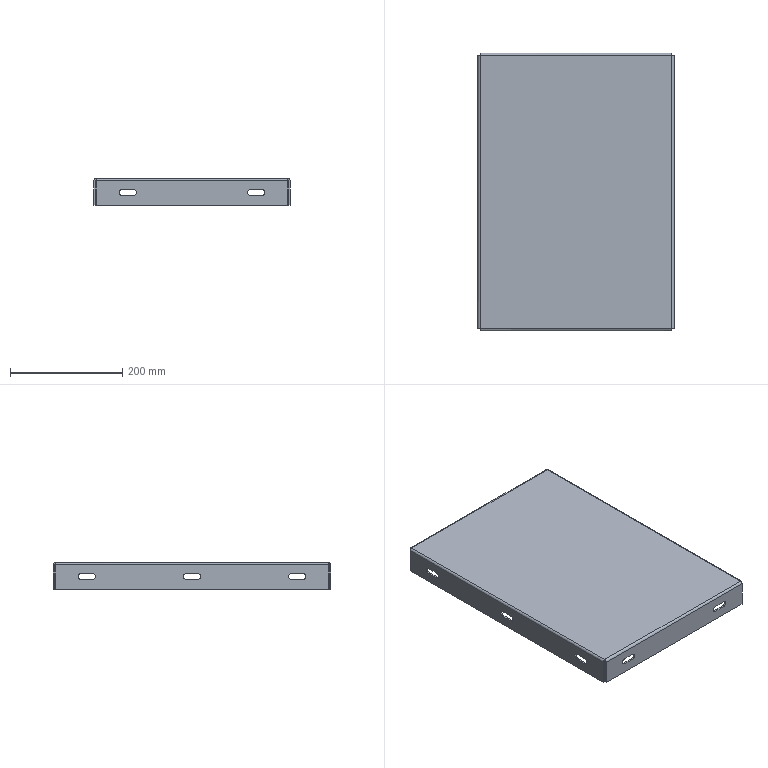Part | NX | features BREP 1 | 1 solid | 78 faces | box 349 x 493.9 x 48 mm | volume 726286 mm3 | plane 42 | cylinder 28 | spline 8 | commonest cylinder face diameters 10.5 x20 2 x4 8 x4